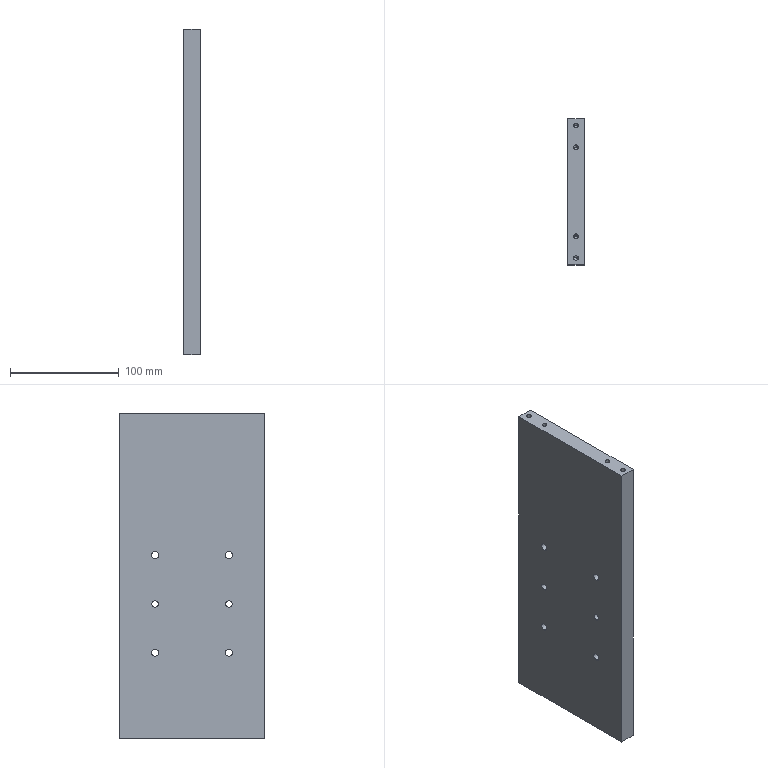Part | SolidWorks | features HoleWzd 7, Extrusion 1, MirrorPattern 1 | 1 solid | 178 faces | box 15 x 134 x 300 mm | volume 594206 mm3 | cylinder 94 | cone 74 | plane 10 | commonest cylinder face diameters 3.3 x44 4.2 x22 4 x8 6.6 x8 11 x8 6 x4